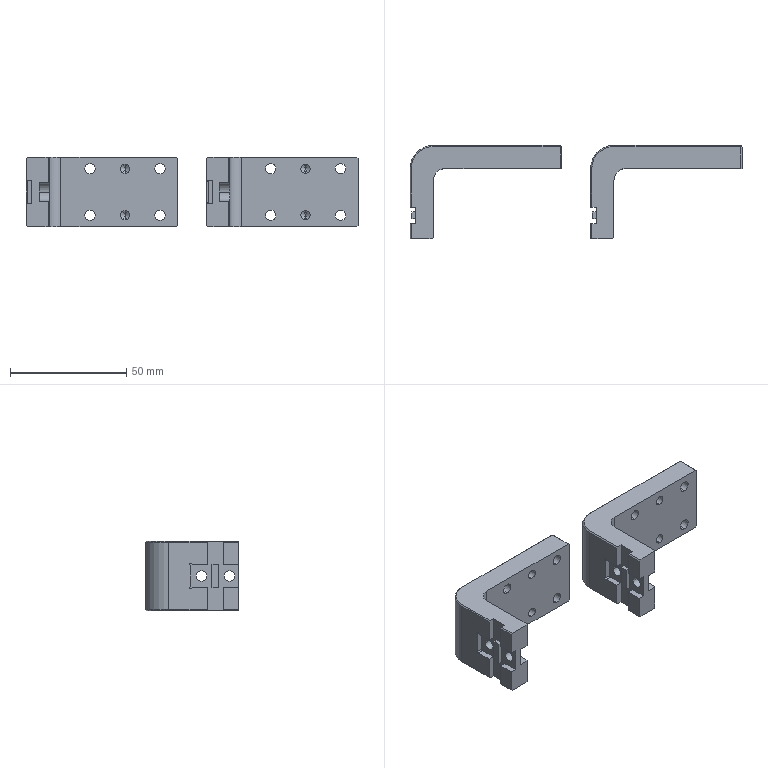NC program | NX | posted with a generic post | part box 142.5 x 40 x 30 mm
Lines 1 to 1042 of 5836:
N10 G17 G21 G94 G90
(ADAPTIVE_MILLING , TOOL : D10)
N12 T15 M6
N14 G54
N16 G17 G0 G90 X-83.926 Y-0.279 B0. C0. S9500 M3
N18 G43 Z30. H15
N20 Z-12.
N22 G94 G1 Z-15. F1000.
N24 X-83.203 Y-0.599 F3500.
N26 X-82.47 Y-0.896
N28 G3 X-81.279 Y-0.279 R1.015
N30 X-80.838 Y2.955 R11.435
N32 X-80.748 Y23.017 R914.738
N34 G2 X-77.811 Y27.631 R5.917
N36 X-72.413 Y29.25 R12.356
N38 X-63.231 Y29.488 R106.897
N40 G1 X-60.169 Y29.491
N42 X-43.794
N44 X74.081
N46 X74.206 Y29.489
N48 X74.331 Y29.484
N50 X74.393 Y29.48
N52 G2 X79.013 Y26.336 R6.013
N54 X80.537 Y20.778 R13.118
N56 X80.739 Y11.407 R130.093
N58 G1 X80.741 Y7.532
N60 X80.742 Y-22.843
N62 X80.741 Y-22.905
N64 X80.737 Y-23.03
N66 X80.73 Y-23.155
N68 X80.719 Y-23.279
N70 G2 X77.519 Y-27.799 R6.086
N72 X72.199 Y-29.269 R13.006
N74 X61.955 Y-29.489 R132.714
N76 G1 X56.955 Y-29.491
N78 X-74.108
N80 X-74.17
N82 X-74.295 Y-29.486
N84 X-74.42 Y-29.478
N86 X-74.544 Y-29.467
N88 G2 X-79.057 Y-26.257 R6.096
N90 X-80.544 Y-20.686 R13.372
N92 X-80.74 Y-10.503 R147.637
N94 X-80.695 Y-1.754 R243.877
N96 G3 X-80.264 Y10.734 R128.976
N98 G2 X-80.229 Y21.295 R692.554
N100 X-76.054 Y27.215 R7.498
N102 X-70.165 Y28.744 R15.462
N104 X-60.233 Y28.982 R127.918
N106 G1 X-57.045 Y28.985
N108 X-44.42 Y28.986
N110 X71.892
N112 X72.017 Y28.985
N114 X72.204 Y28.979
N116 X72.329 Y28.974
N118 G2 X78.362 Y24.976 R7.412
N120 X79.98 Y19.05 R14.976
N122 X80.232 Y9.432 R117.954
N124 G1 X80.235 Y6.744
N126 X80.236 Y-0.381
N128 X80.237 Y-20.631
N130 X80.234 Y-20.818
N132 X80.23 Y-20.943
N134 X80.224 Y-21.068
N136 G2 X76.124 Y-27.167 R7.449
N138 X70.247 Y-28.734 R15.214
N140 X61.003 Y-28.98 R113.17
N142 G1 X58.503 Y-28.984
N144 X52.878 Y-28.986
N146 X-8.122
N148 X-8.435 Y-28.987
N150 X-8.997
N152 X-9.31 Y-28.988
N154 X-11.497 Y-28.987
N156 X-11.81 Y-28.988
N158 X-13.997 Y-28.987
N160 X-14.31 Y-28.988
N162 X-16.497 Y-28.987
N164 X-16.81 Y-28.988
N166 X-18.997 Y-28.987
N168 X-19.31 Y-28.988
N170 X-21.497 Y-28.987
N172 X-21.81 Y-28.988
N174 X-23.997 Y-28.987
N176 X-24.31 Y-28.988
N178 X-26.497 Y-28.987
N180 X-26.81 Y-28.988
N182 X-28.997 Y-28.987
N184 X-29.31 Y-28.988
N186 X-31.497 Y-28.987
N188 X-31.81 Y-28.988
N190 X-33.997 Y-28.987
N192 X-34.31 Y-28.988
N194 X-36.497 Y-28.987
N196 X-36.81 Y-28.988
N198 X-38.997 Y-28.987
N200 X-39.31 Y-28.988
N202 X-41.497 Y-28.987
N204 X-41.81 Y-28.988
N206 X-43.997 Y-28.987
N208 X-44.31 Y-28.988
N210 X-46.497 Y-28.987
N212 X-46.81 Y-28.988
N214 X-48.997 Y-28.987
N216 X-49.31 Y-28.988
N218 X-51.497 Y-28.987
N220 X-51.81 Y-28.988
N222 X-53.997 Y-28.987
N224 X-54.31 Y-28.988
N226 X-56.497 Y-28.987
N228 X-56.81 Y-28.988
N230 X-58.997 Y-28.987
N232 X-59.31 Y-28.988
N234 X-61.497 Y-28.987
N236 X-61.81 Y-28.988
N238 X-63.997 Y-28.987
N240 X-64.31 Y-28.988
N242 X-66.497 Y-28.987
N244 X-66.81 Y-28.988
N246 X-68.997 Y-28.987
N248 X-69.31 Y-28.988
N250 X-71.497 Y-28.987
N252 X-71.872 Y-28.988
N254 X-72.06 Y-28.986
N256 X-72.185 Y-28.983
N258 X-72.309 Y-28.977
N260 X-72.496 Y-28.964
N262 G2 X-78.413 Y-24.885 R7.466
N264 X-79.99 Y-18.946 R15.251
N266 X-80.231 Y-9.89 R114.274
N268 X-79.917 Y2.29 R141.776
N270 G3 X-79.752 Y19.225 R537.495
N272 G2 X-74.752 Y26.717 R8.467
N274 X-68.221 Y28.257 R18.051
N276 X-56.351 Y28.478 R179.687
N278 G1 X-51.163 Y28.48
N280 X70.024
N282 X70.274 Y28.478
N284 X70.462 Y28.473
N286 X70.649 Y28.466
N288 X70.774 Y28.459
N290 G2 X77.879 Y23.659 R8.408
N292 X79.495 Y17.086 R17.506
N294 X79.727 Y6.779 R147.07
N296 G1 X79.73 Y3.654
N298 X79.731 Y-5.596
N300 Y-18.784
N302 X79.728 Y-19.034
N304 X79.723 Y-19.221
N306 X79.716 Y-19.409
N308 G2 X74.787 Y-26.689 R8.439
N310 X68.574 Y-28.224 R17.387
N312 X58.58 Y-28.475 R130.867
N314 G1 X55.83 Y-28.479
N316 X49.58 Y-28.481
N318 X-5.92
N320 X-6.482 Y-28.483
N322 X-6.982 Y-28.484
N324 X-7.357 Y-28.485
N326 X-8.107 Y-28.484
N328 X-8.42 Y-28.485
N330 X-9.607
N332 X-10.545
N334 X-10.982 Y-28.486
N336 X-12.045 Y-28.485
N338 X-12.92
N340 X-13.232 Y-28.486
N342 X-14.42 Y-28.485
N344 X-14.92 Y-28.486
N346 X-16.92 Y-28.485
N348 X-17.42
N350 X-18.482 Y-28.484
N352 X-18.795 Y-28.485
N354 X-19.92
N356 X-20.857 Y-28.484
N358 X-21.17 Y-28.486
N360 X-21.982 Y-28.485
N362 X-22.42 Y-28.486
N364 X-24.482 Y-28.485
N366 X-24.982
N368 X-26.107 Y-28.484
N370 X-26.545 Y-28.485
N372 X-28.17
N374 X-28.482 Y-28.486
N376 X-29.545 Y-28.485
N378 X-30.67
N380 X-30.982 Y-28.486
N382 X-31.982 Y-28.485
N384 X-32.42 Y-28.486
N386 X-34.482 Y-28.485
N388 X-34.982
N390 X-36.107 Y-28.484
N392 X-36.545 Y-28.485
N394 X-38.232
N396 X-38.545 Y-28.486
N398 X-39.545 Y-28.485
N400 X-40.357
N402 X-40.795 Y-28.486
N404 X-41.982 Y-28.485
N406 X-42.607
N408 X-43.045 Y-28.486
N410 X-43.732 Y-28.485
N412 X-44.107 Y-28.486
N414 X-44.545
N416 X-44.982 Y-28.487
N418 X-46.482 Y-28.485
N420 X-47.607 Y-28.488
N422 X-47.92
N424 X-48.732 Y-28.487
N426 X-49.17 Y-28.488
N428 X-49.482 Y-28.487
N430 X-50.107 Y-28.488
N432 X-50.92 Y-28.487
N434 X-51.357 Y-28.488
N436 X-51.982 Y-28.487
N438 X-52.42
N440 X-52.982 Y-28.486
N442 X-53.357 Y-28.487
N444 X-54.357 Y-28.486
N446 X-54.795 Y-28.487
N448 X-55.295 Y-28.486
N450 X-55.67 Y-28.487
N452 X-56.92 Y-28.485
N454 X-57.357 Y-28.486
N456 X-57.982 Y-28.485
N458 X-58.42 Y-28.486
N460 X-59.482 Y-28.485
N462 X-60.67
N464 X-61.107 Y-28.486
N466 X-61.92 Y-28.485
N468 X-62.42 Y-28.487
N470 X-64.295 Y-28.484
N472 X-64.795 Y-28.485
N474 X-65.607
N476 X-65.92 Y-28.486
N478 X-67.045 Y-28.485
N480 X-67.92
N482 X-68.232 Y-28.486
N484 G2 X-72.033 Y-28.302 R19.959
N486 X-78.079 Y-23.25 R8.597
N488 X-79.518 Y-16.819 R18.703
N490 X-79.419 Y2.483 R179.814
N492 G3 X-79.243 Y17.981 R776.744
N494 G2 X-73.65 Y26.199 R9.225
N496 X-66.923 Y27.736 R19.589
N498 X-55.303 Y27.972 R173.807
N500 G1 X-51.365 Y27.975
N502 X-24.678
N504 X68.322
N506 X68.635 Y27.973
N508 X68.885 Y27.968
N510 X69.135 Y27.961
N512 G2 X77.438 Y22.402 R9.208
N514 X78.962 Y15.927 R19.081
N516 X79.219 Y5.808 R137.24
N518 G1 X79.223 Y3.308
N520 X79.225 Y-1.567
N522 X79.226 Y-17.13
N524 X79.224 Y-17.38
N526 X79.217 Y-17.692
N528 X79.208 Y-17.942
N530 G2 X73.656 Y-26.184 R9.199
N532 X66.87 Y-27.736 R19.47
N534 X54.562 Y-27.973 R185.441
N536 G1 X49.625 Y-27.975
N538 X-3.813 Y-27.976
N540 X-4.25 Y-27.977
N542 X-4.688 Y-27.978
N544 X-6.875 Y-27.98
N546 X-12.813 Y-27.987
N548 X-13.25 Y-27.988
N550 X-13.938 Y-27.986
N552 X-14.438 Y-27.987
N554 X-14.813 Y-27.986
N556 X-15.313 Y-27.985
N558 X-15.688
N560 X-16.125
N562 X-16.5
N564 X-17.
N566 X-18.813 Y-27.983
N568 X-19.25
N570 X-19.938
N572 X-20.438 Y-27.984
N574 X-21.125 Y-27.983
N576 X-21.563 Y-27.984
N578 X-22.688 Y-27.983
N580 X-23.313 Y-27.982
N582 X-23.625 Y-27.983
N584 X-25.063
N586 X-26.25 Y-27.982
N588 X-26.75 Y-27.983
N590 X-28.25 Y-27.982
N592 X-29. Y-27.984
N594 X-29.438
N596 X-30.5 Y-27.987
N598 X-31.5 Y-27.984
N600 X-31.938 Y-27.985
N602 X-32.5
N604 X-33.5 Y-27.983
N606 X-34. Y-27.984
N608 X-34.375
N610 X-35.75 Y-27.986
N612 X-36.313 Y-27.985
N614 X-37.313 Y-27.984
N616 X-38.25
N618 X-38.688
N620 X-39.25
N622 X-39.75
N624 X-40.125
N626 X-40.875 Y-27.986
N628 X-41.813 Y-27.984
N630 X-43.875 Y-27.983
N632 X-45.813 Y-27.987
N634 X-46.625 Y-27.986
N636 X-47.5
N638 X-47.938
N640 X-48.813 Y-27.985
N642 X-49.938
N644 X-50.875
N646 X-51.313
N648 X-52.25 Y-27.984
N650 X-52.688 Y-27.985
N652 X-53.313
N654 X-53.813
N656 X-54.813 Y-27.984
N658 X-55.313
N660 X-55.938
N662 X-56.438
N664 X-57.313 Y-27.983
N666 X-57.813 Y-27.984
N668 X-58.563 Y-27.983
N670 X-59. Y-27.984
N672 X-59.813 Y-27.983
N674 X-60.313 Y-27.984
N676 X-60.938 Y-27.983
N678 X-61.375 Y-27.984
N680 X-62.375 Y-27.983
N682 X-63.438
N684 G2 X-69.998 Y-27.905 R92.562
N686 X-77.406 Y-22.472 R9.175
N688 X-78.982 Y-15.692 R19.296
N690 X-79.005 Y0.299 R140.714
N692 G3 X-78.752 Y16.484 R540.74
N694 G2 X-72.498 Y25.748 R9.908
N696 X-65.501 Y27.237 R21.575
N698 X-52.068 Y27.468 R220.389
N700 G1 X-45.943 Y27.47
N702 X66.807
N704 X67.244 Y27.466
N706 X67.557 Y27.461
N708 X67.807 Y27.453
N710 G2 X76.98 Y21.262 R9.857
N712 X78.474 Y14.394 R21.28
N714 X78.716 Y3.086 R172.526
N716 G1 X78.719 Y-0.164
N718 X78.72 Y-8.789
N720 Y-15.601
N722 X78.718 Y-15.914
N724 X78.712 Y-16.289
N726 X78.705 Y-16.539
N728 G2 X72.585 Y-25.697 R9.847
N730 X65.848 Y-27.208 R20.779
N732 X54.729 Y-27.465 R158.332
N734 G1 X51.541 Y-27.468
N736 X43.979 Y-27.47
N738 X-1.646
N740 X-2.146 Y-27.472
N742 X-2.646
N744 X-4.209 Y-27.474
N746 X-6.334 Y-27.476
N748 X-11.271 Y-27.48
N750 X-15.084 Y-27.486
N752 X-15.959
N754 X-16.709 Y-27.484
N756 X-17.271 Y-27.485
N758 X-19.396 Y-27.486
N760 X-20.021
N762 X-20.459 Y-27.485
N764 X-21.084
N766 X-21.521
N768 X-22.396 Y-27.486
N770 X-22.959 Y-27.484
N772 X-23.459
N774 X-25.834 Y-27.48
N776 X-27.959 Y-27.481
N778 X-29.834 Y-27.485
N780 X-30.334 Y-27.484
N782 X-30.959 Y-27.483
N784 X-31.459 Y-27.484
N786 X-33.396 Y-27.487
N788 X-34.584 Y-27.488
N790 X-35.084 Y-27.487
N792 X-36.896 Y-27.488
N794 X-37.334 Y-27.487
N796 X-37.771 Y-27.486
N798 X-38.146
N800 X-39.021 Y-27.487
N802 X-39.646
N804 X-40.084 Y-27.486
N806 X-40.396
N808 X-40.834 Y-27.485
N810 X-41.396 Y-27.486
N812 X-42.021 Y-27.484
N814 X-43.771 Y-27.488
N816 X-44.209 Y-27.487
N818 X-44.834 Y-27.488
N820 X-45.459 Y-27.487
N822 X-45.896
N824 X-46.459 Y-27.485
N826 X-47.584 Y-27.487
N828 X-48.396
N830 X-48.896 Y-27.486
N832 X-49.334 Y-27.487
N834 X-49.709 Y-27.486
N836 X-51.021 Y-27.488
N838 X-51.959 Y-27.487
N840 X-56.209
N842 G2 X-68.208 Y-27.445 R710.736
N844 X-76.966 Y-21.301 R9.836
N846 X-78.492 Y-14.186 R21.566
N848 X-78.476 Y1.056 R148.379
N850 G3 X-78.251 Y15.366 R790.349
N852 G2 X-75.595 Y22.462 R10.638
N854 X-69.062 Y26.046 R12.769
N856 X-61.37 Y26.872 R38.081
N858 X-45.121 Y26.964 R772.922
N860 G1 X7.754 Y26.965
N862 X8.067 Y26.966
N864 X8.629
N866 X8.942 Y26.967
N868 X11.129 Y26.966
N870 X11.442 Y26.967
N872 X13.629 Y26.966
N874 X13.942 Y26.967
N876 X16.129 Y26.966
N878 X16.442 Y26.967
N880 X18.629 Y26.966
N882 X18.942 Y26.967
N884 X21.129 Y26.966
N886 X21.442 Y26.967
N888 X23.629 Y26.966
N890 X23.942 Y26.967
N892 X26.129 Y26.966
N894 X26.442 Y26.967
N896 X28.629 Y26.966
N898 X28.942 Y26.967
N900 X31.129 Y26.966
N902 X31.442 Y26.967
N904 X33.629 Y26.966
N906 X33.942 Y26.967
N908 X36.129 Y26.966
N910 X36.442 Y26.967
N912 X38.629 Y26.966
N914 X38.942 Y26.967
N916 X41.129 Y26.966
N918 X41.442 Y26.967
N920 X43.629 Y26.966
N922 X43.942 Y26.967
N924 X46.129 Y26.966
N926 X46.442 Y26.967
N928 X48.629 Y26.966
N930 X48.942 Y26.967
N932 X51.129 Y26.966
N934 X51.442 Y26.967
N936 X53.629 Y26.966
N938 X53.942 Y26.967
N940 X56.129 Y26.966
N942 X56.442 Y26.967
N944 X58.629 Y26.966
N946 X58.942 Y26.967
N948 X61.129 Y26.966
N950 X61.442 Y26.967
N952 G2 X67.689 Y26.879 R92.418
N954 X76.343 Y20.598 R10.251
N956 X77.933 Y13.624 R21.295
N958 X78.211 Y1.131 R172.806
N960 X78.176 Y-15.806 R907.126
N962 X71.628 Y-25.19 R10.342
N964 X64.385 Y-26.72 R22.52
N966 X53.827 Y-26.958 R163.385
N968 G1 X51.077 Y-26.962
N970 X45.765 Y-26.964
N972 X0.64 Y-26.965
N974 X0.077 Y-26.967
N976 X-0.423
N978 X-1.673 Y-26.971
N980 X-2.423
N982 X-2.985 Y-26.972
N984 X-4.485 Y-26.976
N986 X-5.048 Y-26.975
N988 X-5.673 Y-26.976
N990 X-6.173
N992 X-6.798 Y-26.977
N994 X-7.235 Y-26.976
N996 X-7.985 Y-26.978
N998 X-8.423
N1000 X-9.235 Y-26.98
N1002 X-9.61 Y-26.979
N1004 X-10.548 Y-26.982
N1006 X-10.923 Y-26.981
N1008 X-12.11 Y-26.984
N1010 X-12.485 Y-26.983
N1012 X-13.173 Y-26.985
N1014 X-13.61
N1016 X-13.923
N1018 X-14.61 Y-26.984
N1020 X-15.11
N1022 X-16.298 Y-26.986
N1024 X-16.86 Y-26.985
N1026 X-17.298 Y-26.986
N1028 X-17.735 Y-26.985
N1030 X-17.985 Y-26.986
N1032 X-18.61 Y-26.984
N1034 X-19.048 Y-26.985
N1036 X-19.548 Y-26.984
N1038 X-20.36 Y-26.986
N1040 X-20.86 Y-26.985
N1042 X-21.735 Y-26.984
N1044 X-22.735 Y-26.982
N1046 X-23.173
N1048 X-23.798 Y-26.981
N1050 X-24.423 Y-26.982
N1052 X-24.86 Y-26.981
N1054 X-27.86 Y-26.986
N1056 X-28.36 Y-26.984
N1058 X-28.735 Y-26.985
N1060 X-28.985 Y-26.984
N1062 X-31.548 Y-26.989
N1064 X-31.923 Y-26.988
N1066 X-32.548 Y-26.989
N1068 X-32.985 Y-26.988
N1070 X-33.735 Y-26.989
N1072 X-34.173 Y-26.988
N1074 X-34.923 Y-26.989
N1076 X-35.673
N1078 X-36.235 Y-26.988
N1080 X-37.485 Y-26.989
N1082 X-37.985
N1084 X-38.36
N1086 X-38.923 Y-26.988
N1088 X-39.36
N1090 X-39.86 Y-26.986
N1092 X-41.61 Y-26.989
N1094 X-42.11
N1096 X-42.673 Y-26.99
N1098 X-43.423 Y-26.988
N1100 X-43.798
N1102 X-44.985 Y-26.986
N1104 X-45.173 Y-26.985
N1106 X-46.235 Y-26.988
N1108 X-46.735 Y-26.987
N1110 X-47.173
N1112 X-47.61
N1114 X-47.923 Y-26.988
N1116 X-48.298 Y-26.987
N1118 X-48.923 Y-26.988
N1120 X-49.423 Y-26.987
N1122 X-49.86 Y-26.988
N1124 X-50.298 Y-26.987
N1126 X-50.985 Y-26.988
N1128 X-51.485 Y-26.987
N1130 X-52.048 Y-26.988
N1132 X-52.61 Y-26.987
N1134 X-53.11 Y-26.988
N1136 X-53.798 Y-26.987
N1138 X-54.235
N1140 X-55.173 Y-26.985
N1142 X-55.548 Y-26.986
N1144 X-57.048 Y-26.983
N1146 X-57.36
N1148 X-58.048 Y-26.982
N1150 X-58.485 Y-26.983
N1152 X-59.235 Y-26.984
N1154 X-60.485 Y-26.982
N1156 X-61.36
N1158 X-61.798
N1160 G2 X-67.981 Y-26.859 R65.177
N1162 X-73.509 Y-24.537 R10.651
N1164 G1 X-73.769 Y-24.43
N1166 X-73.799 Y-24.415
N1168 X-73.827 Y-24.396
N1170 G2 X-76.231 Y-21.365 R5.864
N1172 X-77.959 Y-13.465 R24.366
N1174 X-78.02 Y-0.472 R121.464
N1176 G3 X-77.751 Y14.337 R833.339
N1178 G2 X-75.583 Y21.065 R11.504
N1180 X-69.026 Y25.29 R12.331
N1182 X-61.239 Y26.327 R33.16
N1184 X-44.428 Y26.459 R559.705
N1186 G1 X5.635
N1188 X6.135 Y26.461
N1190 X6.697
N1192 X7.135 Y26.462
N1194 X9.01
N1196 X9.51 Y26.463
N1198 X11.135 Y26.462
N1200 X11.447 Y26.463
N1202 X11.76
N1204 X12.072 Y26.464
N1206 X12.572
N1208 X12.885 Y26.465
N1210 X14.072 Y26.464
N1212 X14.51 Y26.465
N1214 X15.135 Y26.464
N1216 X15.635 Y26.465
N1218 X16.635 Y26.464
N1220 X17.135
N1222 X18.072 Y26.463
N1224 X18.447 Y26.465
N1226 X18.947
N1228 X19.51 Y26.466
N1230 X20.135 Y26.467
N1232 X21.01 Y26.465
N1234 X22.01 Y26.467
N1236 X22.885 Y26.468
N1238 X23.51 Y26.466
N1240 X24.76 Y26.469
N1242 X25.385 Y26.467
N1244 X26.01 Y26.468
N1246 X26.572 Y26.467
N1248 X27.072
N1250 X27.76 Y26.468
N1252 X28.385 Y26.466
N1254 X29.51 Y26.468
N1256 X30.135 Y26.467
N1258 X30.697 Y26.468
N1260 X31.322 Y26.466
N1262 X32.51 Y26.468
N1264 X33.197 Y26.466
N1266 X33.76 Y26.467
N1268 X34.135 Y26.466
N1270 X34.635 Y26.467
N1272 X35.01 Y26.466
N1274 X36.947 Y26.469
N1276 X37.572 Y26.467
N1278 X38.197 Y26.468
N1280 X38.822 Y26.466
N1282 X40.072 Y26.468
N1284 X40.76 Y26.466
N1286 X41.322 Y26.467
N1288 X41.635 Y26.466
N1290 X42.135 Y26.467
N1292 X42.447 Y26.466
N1294 X42.885 Y26.467
N1296 X43.635 Y26.465
N1298 X44.635 Y26.467
N1300 X45.385 Y26.466
N1302 X47.385 Y26.469
N1304 X48.01 Y26.467
N1306 X48.635 Y26.468
N1308 X49.197 Y26.467
N1310 X49.635
N1312 X50.26
N1314 X50.947 Y26.466
N1316 X51.947 Y26.468
N1318 X52.635 Y26.466
N1320 X53.135 Y26.467
N1322 G2 X66.071 Y26.415 R505.878
N1324 X71.334 Y24.987 R12.858
N1326 X75.765 Y21.592 R6.232
N1328 X76.831 Y17.43 R23.171
N1330 X77.658 Y7.165 R59.191
N1332 G1 X77.673 Y6.102
N1334 X77.684 Y5.04
N1336 X77.692 Y3.977
N1338 X77.7 Y2.29
N1340 X77.705 Y-0.023
N1342 X77.708 Y-3.71
N1344 G2 X77.649 Y-15.021 R320.606
N1346 X70.923 Y-24.596 R10.724
N1348 X63.442 Y-26.203 R23.145
N1350 X51.697 Y-26.454 R178.822
N1352 G1 X48.447 Y-26.457
N1354 X41.01 Y-26.459
N1356 X2.76
N1358 X2.26 Y-26.461
N1360 X0.885 Y-26.462
N1362 X-1.365 Y-26.466
N1364 X-1.803 Y-26.468
N1366 X-9.553 Y-26.476
N1368 X-10.053 Y-26.478
N1370 X-11.49 Y-26.479
N1372 X-12.428 Y-26.48
N1374 X-13.053
N1376 X-13.865 Y-26.483
N1378 X-16.803 Y-26.481
N1380 X-17.053 Y-26.482
N1382 X-17.615
N1384 X-17.99 Y-26.483
N1386 X-24.115 Y-26.48
N1388 X-28.615 Y-26.481
N1390 X-29.053 Y-26.483
N1392 X-31.178 Y-26.484
N1394 X-31.74 Y-26.486
N1396 X-32.24 Y-26.485
N1398 X-32.803 Y-26.486
N1400 X-33.49 Y-26.488
N1402 X-33.928 Y-26.487
N1404 X-34.24 Y-26.488
N1406 X-34.865 Y-26.487
N1408 X-35.428 Y-26.488
N1410 X-36.303 Y-26.489
N1412 X-36.803
N1414 X-37.24
N1416 X-37.803 Y-26.487
N1418 X-38.24
N1420 X-38.553
N1422 X-39.553 Y-26.489
N1424 X-40.24 Y-26.49
N1426 X-41.553 Y-26.487
N1428 X-42.678 Y-26.486
N1430 X-44.115 Y-26.488
N1432 X-44.553
N1434 X-45.115
N1436 X-45.615
N1438 X-46.303
N1440 X-46.865 Y-26.489
N1442 X-47.365 Y-26.488
N1444 X-47.865
N1446 X-48.303
N1448 X-50.053 Y-26.49
N1450 X-50.678 Y-26.489
N1452 X-51.115
N1454 X-51.74 Y-26.487
N1456 X-52.178 Y-26.488
N1458 G2 X-66.052 Y-26.429 R576.006
N1460 X-71.161 Y-25.117 R13.12
N1462 G1 X-71.222 Y-25.103
N1464 X-71.236 Y-25.099
N1466 X-71.283 Y-25.096
N1468 X-72.537 Y-24.931
N1470 X-72.569 Y-24.924
N1472 X-72.601 Y-24.913
N1474 X-73.525 Y-24.531
N1476 X-73.827 Y-24.396
N1478 X-74.877 Y-23.579
N1480 X-75.665 Y-22.549
N1482 X-75.68 Y-22.519
N1484 X-76.163 Y-21.351
N1486 X-76.174 Y-21.319
N1488 X-76.181 Y-21.287
N1490 G2 X-77.174 Y-15.625 R180.655
N1492 X-77.577 Y-2.768 R85.896
N1494 G3 X-77.253 Y13.353 R955.982
N1496 G2 X-75.26 Y20.025 R12.286
N1498 X-68.487 Y24.674 R12.396
N1500 X-60.775 Y25.793 R31.936
N1502 X-45.277 Y25.953 R415.916
N1504 G1 X-31.527 Y25.954
N1506 X3.348
N1508 X5.035 Y25.96
N1510 X5.535
N1512 X5.973 Y25.961
N1514 X6.598 Y25.962
N1516 X6.973 Y25.961
N1518 X7.473
N1520 X9.223 Y25.96
N1522 X9.848 Y25.961
N1524 X10.223 Y25.962
N1526 X10.598
N1528 X10.973 Y25.963
N1530 X11.973 Y25.962
N1532 X12.41 Y25.963
N1534 X13.098 Y25.962
N1536 X13.535 Y25.963
N1538 X14.535 Y25.962
N1540 X14.973 Y25.963
N1542 X15.973 Y25.962
N1544 X19.348 Y25.963
N1546 X21.723 Y25.967
N1548 X22.285
N1550 X22.723
N1552 X23.535 Y25.966
N1554 X24.035
N1556 X24.473
N1558 X24.973 Y25.967
N1560 X25.473
N1562 X25.848 Y25.968
N1564 X26.41 Y25.967
N1566 X26.848
N1568 X27.285 Y25.966
N1570 X27.723 Y25.967
N1572 X28.223 Y25.966
N1574 X28.66 Y25.967
N1576 X29.41 Y25.966
N1578 X29.848
N1580 X30.223
N1582 X31.098 Y25.965
N1584 X31.785 Y25.966
N1586 X33.035 Y25.965
N1588 X33.535 Y25.966
N1590 X35.16 Y25.968
N1592 X35.66
N1594 X36.223
N1596 X36.785 Y25.967
N1598 X38.098 Y25.969
N1600 X38.723 Y25.967
N1602 X39.285 Y25.968
N1604 X39.723
N1606 X40.16
N1608 X40.66
N1610 X41.535 Y25.966
N1612 X42.535 Y25.968
N1614 X42.973 Y25.967
N1616 X44.41 Y25.969
N1618 X44.723 Y25.968
N1620 X45.285 Y25.969
N1622 X45.91 Y25.967
N1624 X46.348 Y25.968
N1626 X47.285 Y25.966
N1628 X48.785 Y25.965
N1630 X49.41
N1632 X52.848 Y25.963
N1634 X56.223 Y25.966
N1636 G2 X65.409 Y25.886 R189.812
N1638 X69.321 Y25.101 R19.103
N1640 X71.459 Y24.964 R13.233
N1642 G3 X72.496 Y26.376 R1.012
N1644 G1 X72.326 Y26.763
N1646 X72.141 Y27.143
N1648 G3 X70.951 Y27.535 R1.017
N1650 G1 Z-12.
N1652 G0 Z53.
N1654 X-75.719 Y-26.089
N1656 Z-12.
N1658 G1 Z-15. F1000.
N1660 G2 X-77.049 Y-24.912 R1.012 F3500.
N1662 G1 X-76.211 Y-21.28
N1664 X-76.213 Y-21.039
N1666 G2 X-76.386 Y-18.592 R18.109
N1668 X-77.011 Y-0.622 R114.519
N1670 G1 X-77. Y-0.122
N1672 X-76.98 Y0.69
N1674 X-76.968 Y1.252
N1676 X-76.954 Y1.814
N1678 X-76.891 Y4.814
N1680 X-76.869 Y6.251
N1682 X-76.852 Y7.626
N1684 X-76.844 Y8.126
N1686 X-76.824 Y9.876
N1688 X-76.806 Y10.876
N1690 X-76.795 Y11.376
N1692 X-76.782 Y11.813
N1694 X-76.768 Y12.188
N1696 G2 X-75.163 Y18.609 R13.645
N1698 X-68.495 Y23.885 R12.137
N1700 X-60.887 Y25.224 R28.182
N1702 X-48.579 Y25.443 R234.523
N1704 G1 X-45.016 Y25.447
N1706 X-36.204 Y25.448
N1708 X1.234 Y25.449
N1710 X1.671 Y25.45
N1712 X2.359
N1714 X2.984 Y25.454
N1716 X3.484
N1718 X3.859 Y25.456
N1720 X36.421 Y25.472
N1722 X37.171 Y25.471
N1724 X37.609 Y25.47
N1726 X38.109
N1728 X39.046
N1730 X39.484 Y25.469
N1732 X40.296 Y25.47
N1734 X40.984 Y25.468
N1736 X41.484
N1738 X41.796
N1740 X42.421 Y25.469
N1742 X43.359
N1744 X44.296 Y25.47
N1746 X44.796
N1748 X45.421 Y25.469
N1750 X45.796
N1752 X47.421 Y25.468
N1754 G2 X63.858 Y25.415 R863.363
N1756 X66.611 Y25.1 R27.402
N1758 G1 X69.361
N1760 G3 X70.056 Y26.843 R1.011
N1762 G1 X69.37 Y27.477
N1764 G3 X68.468 Y27.6 R1.025
N1766 G1 Z-12.
N1768 G0 Z53.
N1770 X-78.225 Y-22.895
N1772 Z-12.
N1774 G1 Z-15. F1000.
N1776 G2 X-78.906 Y-20.994 R1.01 F3500.
N1778 G1 X-77.008 Y-20.288
N1780 G3 X-76.35 Y-19.341 R1.02
N1782 X-76.554 Y-9.658 R177.455
N1784 G2 X-76.434 Y2.653 R277.058
N1786 X-76.297 Y11.207 R482.355
N1788 X-74.799 Y17.602 R14.859
N1790 X-69.327 Y22.705 R11.852
N1792 G1 X-68.14 Y23.433
N1794 X-68.068 Y23.47
N1796 X-65.954 Y24.345
N1798 X-65.877 Y24.37
N1800 X-63.652 Y24.905
N1802 X-63.572 Y24.917
N1804 X-61.27 Y25.098
N1806 X-61.23 Y25.1
N1808 X-7.279
N1810 X-7.221 Y25.097
N1812 X-6.909 Y25.075
N1814 G3 X7.464 Y24.961 R349.765
N1816 G1 X7.839 Y24.96
N1818 X9.151 Y24.961
N1820 X9.526 Y24.96
N1822 X10.839 Y24.962
N1824 X11.214 Y24.961
N1826 X12.526 Y24.963
N1828 X13.089 Y24.962
N1830 X14.482 Y24.961
N1832 X16.23 Y25.098
N1834 X16.27 Y25.1
N1836 X66.645
N1838 G3 X67.743 Y26.202 R1.1
N1840 X66.645 Y27.3 R1.1
N1842 G1 X15.11 Y27.293
N1844 X13.11 Z-14.9
N1846 X-5.034 Y27.29
N1848 X-7.034 Z-15.
N1850 G3 X-7.221 Y25.097 R1.101
N1852 G2 X-4.548 Y24.695 R37.43
N1854 G3 X3.758 Y24.468 R89.38
N1856 G1 X4.196 Y24.466
N1858 X5.446 Y24.465
N1860 X5.946 Y24.464
N1862 X7.071
N1864 X8.383 Y24.465
N1866 X8.883
N1868 X9.571
N1870 X10.321 Y24.466
N1872 X11.008 Y24.464
N1874 X11.383
N1876 X11.883 Y24.463
N1878 X11.946 Y24.464
N1880 X12.008 Y24.469
N1882 X12.07 Y24.478
N1884 G2 X14.489 Y24.961 R12.431
N1886 G3 X14.518 Y27.152 R1.1
N1888 G1 X12.518 Y27.149 Z-14.9
N1890 X-4.39 Y27.071
N1892 X-5.026 Y27.073 Z-14.932
N1894 X-5.661 Y27.05 Z-14.964
N1896 G3 X-6.288 Y26.707 Z-15. R1.142
N1898 X-5.838 Y24.928 R1.102
N1900 X-1.376 Y24.098 R13.119
N1902 X10.683 Y24.001 R215.145
N1904 G2 X12.109 Y24.487 R8.789
N1906 G3 X12.572 Y26.389 R1.101
N1908 X11.67 Y26.658 Z-14.952 R1.245
N1910 G1 X10.637 Y26.663 Z-14.9
N1912 X-3.486 Y26.731
N1914 X-4.085 Y26.736 Z-14.93
N1916 X-4.685 Y26.725 Z-14.96
N1918 G3 X-5.37 Y26.347 Z-15. R1.132
N1920 X-4.894 Y24.598 R1.102
N1922 X-1.037 Y23.69 R10.172
N1924 X9.519 Y23.52 R115.367
N1926 G1 X9.58 Y23.536
N1928 X9.6 Y23.539
N1930 X10.813 Y24.042
N1932 G3 X11.306 Y25.67 R1.103
N1934 X10.323 Y26.16 Z-14.943 R1.132
N1936 G1 X9.471 Y26.18 Z-14.9
N1938 X-3.055 Y26.475
N1940 X-4.102 Y26.488 Z-14.952
N1942 G3 X-4.887 Y26.003 Z-15. R1.117
N1944 X-4.554 Y24.465 R1.104
N1946 X-1.457 Y23.387 R6.825
N1948 X5.903 Y23.006 R58.775
N1950 X8.71 Y23.077 R19.316
N1952 G1 X8.769 Y23.097
N1954 X8.828 Y23.119
N1956 X8.869 Y23.132
N1958 X9.36 Y23.433
N1960 X9.432 Y23.47
N1962 X9.605 Y23.541
N1964 G3 X10.133 Y25.114 R1.103
N1966 X9.051 Y25.664 Z-14.936 R1.183
N1968 G1 X8.329 Y25.695 Z-14.9
N1970 X-2.54 Y26.158
N1972 X-3.083 Y26.184 Z-14.927
N1974 X-3.628 Y26.189 Z-14.955
N1976 G3 X-4.388 Y25.736 Z-15. R1.127
N1978 X-4.078 Y24.166 R1.104
N1980 X-0.583 Y22.918 R7.537
N1982 X7.712 Y22.584 R48.541
N1984 X8.905 Y23.154 R2.878
N1986 X9.31 Y24.592 R1.106
N1988 X8.292 Y25.195 Z-14.938 R1.124
N1990 G1 X7.54 Y25.234 Z-14.9
N1992 X-1.873 Y25.714
N1994 X-2.913 Y25.755 Z-14.952
N1996 G3 X-3.714 Y25.286 Z-15. R1.117
N1998 X-3.496 Y23.8 R1.104
N2000 X-0.97 Y22.666 R5.286
N2002 X7.115 Y22.154 R31.279
N2004 X8.179 Y22.709 R3.558
N2006 X8.601 Y24.113 R1.106
N2008 X7.599 Y24.751 Z-14.937 R1.124
N2010 G1 X6.854 Y24.811 Z-14.9
N2012 X-1.629 Y25.489
N2014 X-2.657 Y25.559 Z-14.952
N2016 G3 X-3.477 Y25.104 Z-15. R1.117
N2018 X-3.362 Y23.684 R1.106
N2020 X-0.87 Y22.338 R4.83
N2022 X6.448 Y21.725 R23.333
N2024 X7.462 Y22.27 R1.964
N2026 X7.896 Y23.647 R1.106
N2028 X6.908 Y24.312 Z-14.937 R1.124
N2030 G1 X6.168 Y24.388 Z-14.9
N2032 X-1.292 Y25.157
N2034 X-2.322 Y25.251 Z-14.952
N2036 G3 X-3.15 Y24.818 Z-15. R1.117
N2038 X-3.052 Y23.375 R1.106
N2040 X-0.354 Y21.894 R5.215
N2042 X5.962 Y21.326 R18.1
N2044 X7.055 Y21.944 R1.917
N2046 X7.343 Y23.234 R1.108
N2048 X6.379 Y23.884 Z-14.939 R1.126
N2050 G1 X5.607 Y23.979 Z-14.9
N2052 X-0.915 Y24.783
N2054 X-1.946 Y24.899 Z-14.952
N2056 G3 X-2.781 Y24.485 Z-15. R1.117
N2058 X-2.699 Y23.021 R1.106
N2060 X-0.089 Y21.51 R5.073
N2062 X5.533 Y20.944 R14.463
N2064 X6.611 Y21.564 R1.933
N2066 X6.906 Y22.838 R1.108
N2068 X5.956 Y23.503 Z-14.939 R1.126
N2070 G1 X5.183 Y23.615 Z-14.9
N2072 X-0.589 Y24.444
N2074 X-1.625 Y24.581 Z-14.952
N2076 G3 X-2.464 Y24.19 Z-15. R1.117
N2078 X-2.483 Y22.795 R1.106
N2080 X-0.445 Y21.337 R3.895
N2082 X5.138 Y20.578 R12.045